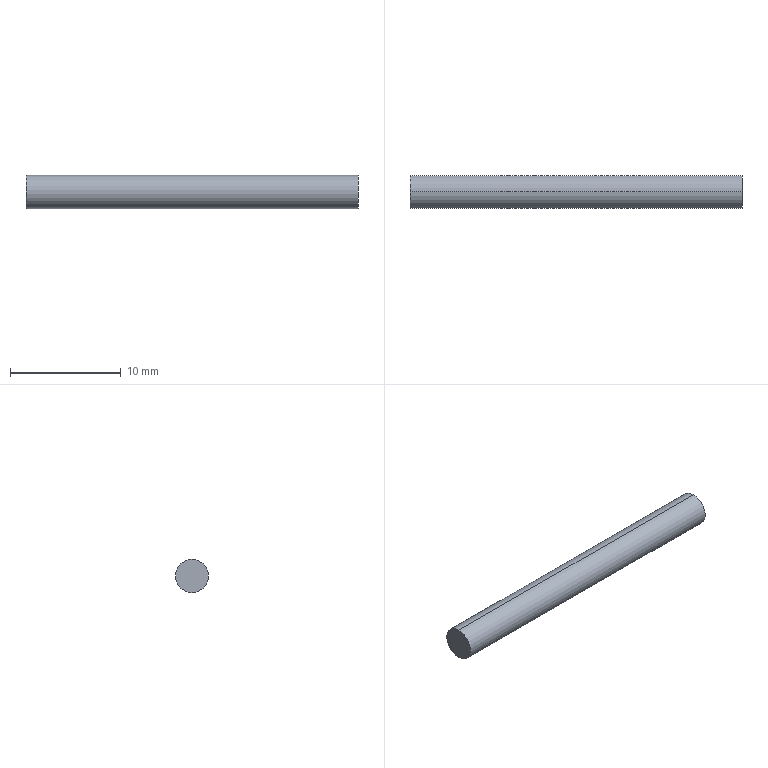Part | SolidWorks | features Revolution 1 | 1 solid | 4 faces | box 30 x 3 x 3 mm | volume 212.058 mm3 | cylinder 2 | plane 2 | commonest cylinder face diameters 3 x2
STEP:
#1=CARTESIAN_POINT('',(30.,0.,1.5));
#2=VERTEX_POINT('',#1);
#3=CARTESIAN_POINT('',(30.,0.,-1.5));
#4=VERTEX_POINT('',#3);
#5=CARTESIAN_POINT('',(30.,0.,0.));
#6=DIRECTION('',(-1.,0.,0.));
#7=DIRECTION('',(0.,0.,1.));
#8=AXIS2_PLACEMENT_3D('',#5,#6,#7);
#9=CIRCLE('',#8,1.5);
#10=EDGE_CURVE('',#2,#4,#9,.T.);
#11=ORIENTED_EDGE('',*,*,#10,.T.);
#12=CARTESIAN_POINT('',(0.,0.,-1.5));
#13=VERTEX_POINT('',#12);
#14=CARTESIAN_POINT('',(0.,0.,-1.5));
#15=DIRECTION('',(-1.,0.,0.));
#16=VECTOR('',#15,1000.);
#17=LINE('',#14,#16);
#18=EDGE_CURVE('',#4,#13,#17,.T.);
#19=ORIENTED_EDGE('',*,*,#18,.T.);
#20=CARTESIAN_POINT('',(0.,0.,1.5));
#21=VERTEX_POINT('',#20);
#22=CARTESIAN_POINT('',(0.,0.,0.));
#23=DIRECTION('',(-1.,0.,0.));
#24=DIRECTION('',(0.,0.,1.));
#25=AXIS2_PLACEMENT_3D('',#22,#23,#24);
#26=CIRCLE('',#25,1.5);
#27=EDGE_CURVE('',#21,#13,#26,.T.);
#28=ORIENTED_EDGE('',*,*,#27,.F.);
#29=CARTESIAN_POINT('',(0.,0.,1.5));
#30=DIRECTION('',(-1.,0.,0.));
#31=VECTOR('',#30,1000.);
#32=LINE('',#29,#31);
#33=EDGE_CURVE('',#2,#21,#32,.T.);
#34=ORIENTED_EDGE('',*,*,#33,.F.);
#35=EDGE_LOOP('',(#11,#19,#28,#34));
#36=FACE_OUTER_BOUND('',#35,.T.);
#37=CARTESIAN_POINT('',(0.,0.,0.));
#38=DIRECTION('',(-1.,0.,0.));
#39=DIRECTION('',(0.,0.,1.));
#40=AXIS2_PLACEMENT_3D('',#37,#38,#39);
#41=CYLINDRICAL_SURFACE('',#40,1.5);
#42=ADVANCED_FACE('',(#36),#41,.T.);
#43=ORIENTED_EDGE('',*,*,#10,.F.);
#44=CARTESIAN_POINT('',(30.,0.,0.));
#45=DIRECTION('',(-1.,0.,0.));
#46=DIRECTION('',(0.,0.,1.));
#47=AXIS2_PLACEMENT_3D('',#44,#45,#46);
#48=CIRCLE('',#47,1.5);
#49=EDGE_CURVE('',#4,#2,#48,.T.);
#50=ORIENTED_EDGE('',*,*,#49,.F.);
#51=EDGE_LOOP('',(#43,#50));
#52=FACE_OUTER_BOUND('',#51,.T.);
#53=CARTESIAN_POINT('',(30.,0.,0.));
#54=DIRECTION('',(-1.,0.,0.));
#55=DIRECTION('',(0.,0.,1.));
#56=AXIS2_PLACEMENT_3D('',#53,#54,#55);
#57=PLANE('',#56);
#58=ADVANCED_FACE('',(#52),#57,.F.);
#59=ORIENTED_EDGE('',*,*,#18,.F.);
#60=ORIENTED_EDGE('',*,*,#49,.T.);
#61=ORIENTED_EDGE('',*,*,#33,.T.);
#62=CARTESIAN_POINT('',(0.,0.,0.));
#63=DIRECTION('',(-1.,0.,0.));
#64=DIRECTION('',(0.,0.,1.));
#65=AXIS2_PLACEMENT_3D('',#62,#63,#64);
#66=CIRCLE('',#65,1.5);
#67=EDGE_CURVE('',#13,#21,#66,.T.);
#68=ORIENTED_EDGE('',*,*,#67,.F.);
#69=EDGE_LOOP('',(#59,#60,#61,#68));
#70=FACE_OUTER_BOUND('',#69,.T.);
#71=CARTESIAN_POINT('',(0.,0.,0.));
#72=DIRECTION('',(-1.,0.,0.));
#73=DIRECTION('',(0.,0.,1.));
#74=AXIS2_PLACEMENT_3D('',#71,#72,#73);
#75=CYLINDRICAL_SURFACE('',#74,1.5);
#76=ADVANCED_FACE('',(#70),#75,.T.);
#77=ORIENTED_EDGE('',*,*,#27,.T.);
#78=ORIENTED_EDGE('',*,*,#67,.T.);
#79=EDGE_LOOP('',(#77,#78));
#80=FACE_OUTER_BOUND('',#79,.T.);
#81=CARTESIAN_POINT('',(0.,0.,0.));
#82=DIRECTION('',(1.,0.,0.));
#83=DIRECTION('',(0.,0.,-1.));
#84=AXIS2_PLACEMENT_3D('',#81,#82,#83);
#85=PLANE('',#84);
#86=ADVANCED_FACE('',(#80),#85,.F.);
#87=CLOSED_SHELL('',(#42,#58,#76,#86));
#88=MANIFOLD_SOLID_BREP('',#87);
#89=CARTESIAN_POINT('',(0.,0.,0.));
#90=DIRECTION('',(0.,0.,1.));
#91=DIRECTION('',(1.,0.,0.));
#92=AXIS2_PLACEMENT_3D('',#89,#90,#91);
#93=(LENGTH_UNIT()NAMED_UNIT(*)SI_UNIT(.MILLI.,.METRE.));
#94=UNCERTAINTY_MEASURE_WITH_UNIT(LENGTH_MEASURE(0.00001),#93,'','');
#95=(NAMED_UNIT(*)PLANE_ANGLE_UNIT()SI_UNIT($,.RADIAN.));
#96=(NAMED_UNIT(*)SI_UNIT($,.STERADIAN.)SOLID_ANGLE_UNIT());
#97=(GEOMETRIC_REPRESENTATION_CONTEXT(3)GLOBAL_UNCERTAINTY_ASSIGNED_CONTEXT((#94))GLOBAL_UNIT_ASSIGNED_CONTEXT((#93,#95,#96))REPRESENTATION_CONTEXT('',''));
#98=ADVANCED_BREP_SHAPE_REPRESENTATION('',(#88,#92),#97);